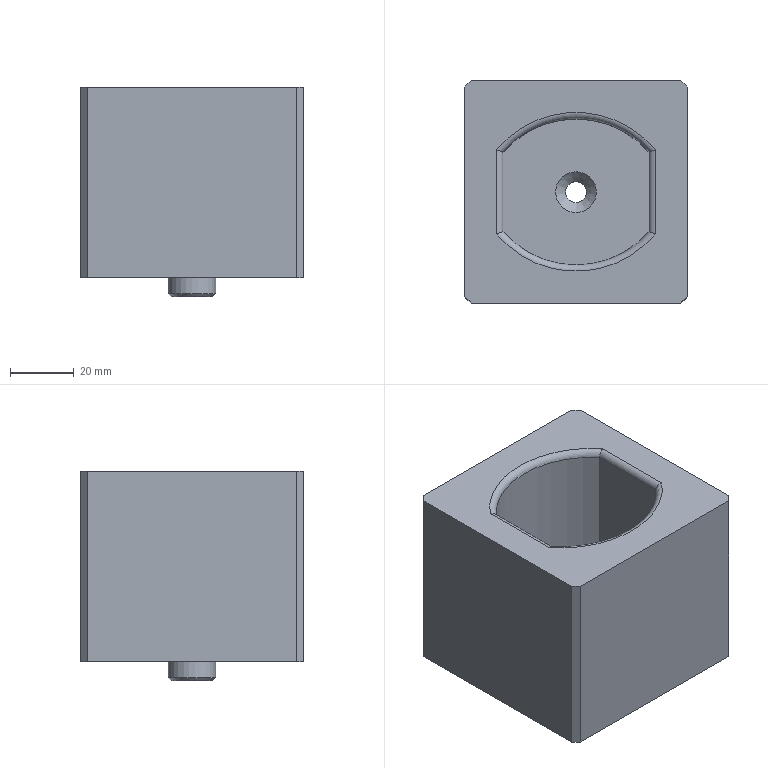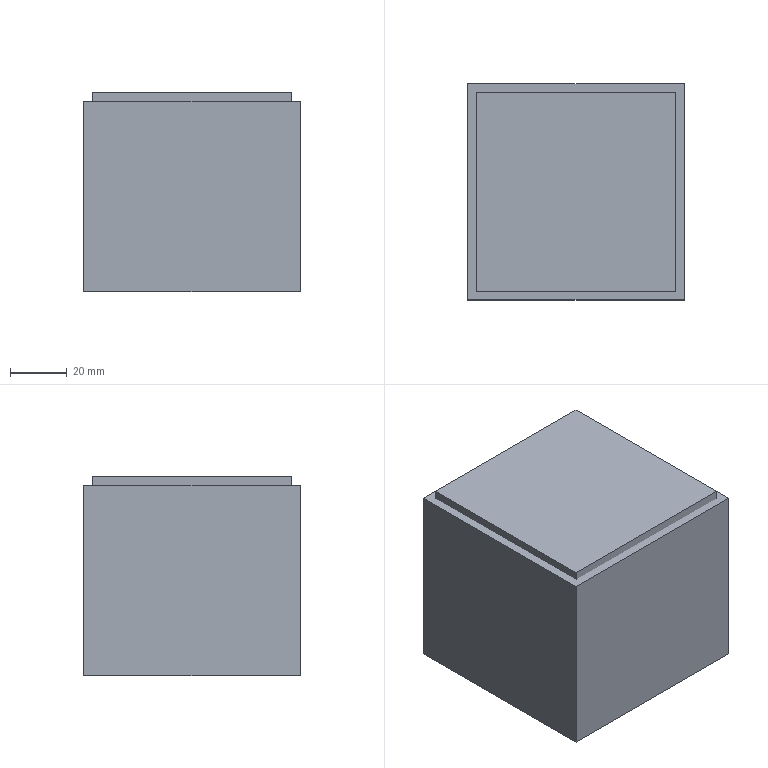CAM job | NX | 3-axis milling, drilling | part box 70 x 70 x 66 mm | stock box 76 x 76 x 70 mm
Tools:
number,name,description,diameter,corner_radius,flute_length,length,flutes
1,D63,Milling Tool-5 Parameters,63.0,0.0,50.0,75.0,2
6,D8A45,Milling Tool-5 Parameters,8.0,0.0,50.0,75.0,2
16,6.6ZT,Drilling Tool,6.6,0.0,35.0,50.0,2
22,D16,Milling Tool-5 Parameters,16.0,0.0,50.0,75.0,2
4,D10,Milling Tool-5 Parameters,10.0,0.0,50.0,75.0,2
18,14.0ZT,Milling Tool-5 Parameters,14.0,0.0,50.0,75.0,2
23,D6R3,Milling Tool-5 Parameters,6.0,3.0,50.0,75.0,2
Operations:
program,operation,operation_type,tool,method,geometry_group,spindle_rpm,surface_speed,feed_per_tooth,feed_cut,feed_plunge,cut_length_mm,path_length_mm,cut_time_min,machine_time_min
1,FLOOR_WALL,VolumeBased25DMillingOperation,D63,METHOD,A,6500.0,1286.0,0.1923,2500.0,100.0,479.797,533.797,0.1919,0.1973
1,DRILLING,Operation,D8A45,METHOD,A,5000.0,0.0,0.0,250.0,0.0,6.4,72.8,0.0256,0.0322
1,DRILLING_COPY,Operation,6.6ZT,METHOD,A,2000.0,41.0,0.0625,250.0,0.0,17.983,95.966,0.0719,0.0797
1,ZLEVEL_PROFILE,ZLevelMilling,D16,METHOD,A,7500.0,376.0,0.1667,2500.0,1000.0,21655.545,21778.745,8.69,8.702
1,ZLEVEL_PROFILE_COPY,ZLevelMilling,D16,METHOD,A,7500.0,376.0,0.0567,850.0,1000.0,1348.483,1540.044,1.583,1.602
1,FLOOR_WALL_1,VolumeBased25DMillingOperation,D10,METHOD,A,7500.0,235.0,0.1667,2500.0,1000.0,6035.627,6237.015,2.448,2.469
1,FLOOR_WALL_1_COPY,VolumeBased25DMillingOperation,D10,METHOD,A,7500.0,235.0,0.0667,1000.0,1000.0,1006.102,1280.289,1.006,1.036
1,PLANAR_MILL,PlanarMilling,D8A45,METHOD,A,7500.0,188.0,0.0833,1250.0,100.0,64.266,121.266,0.0514,0.0571
1,PLANAR_MILL_COPY,PlanarMilling,D8A45,METHOD,A,7500.0,188.0,0.0833,1250.0,100.0,297.482,366.482,0.238,0.2449
2,FLOOR_WALL_COPY,VolumeBased25DMillingOperation,D63,METHOD,B,6500.0,1286.0,0.1923,2500.0,100.0,1823.188,2465.31,0.7293,0.7935
2,ZLEVEL_PROFILE_COPY_1_COPY,ZLevelMilling,D16,METHOD,B,7500.0,376.0,0.1667,2500.0,1000.0,3207.253,3319.303,1.31,1.322
2,ZLEVEL_PROFILE_COPY_1,ZLevelMilling,D16,METHOD,B,7500.0,376.0,0.1667,2500.0,1000.0,5699.6,5811.65,2.307,2.318
2,ZLEVEL_PROFILE_COPY_COPY,ZLevelMilling,D10,METHOD,B,7500.0,376.0,0.0567,850.0,1000.0,784.078,951.443,0.9179,0.9347
2,FLOOR_WALL_1_COPY_COPY,VolumeBased25DMillingOperation,D10,METHOD,B,7500.0,235.0,0.0667,1000.0,1000.0,344.38,511.38,0.3444,0.3611
2,PLANAR_MILL_COPY_COPY,PlanarMilling,D8A45,METHOD,B,7500.0,188.0,0.0833,1250.0,100.0,297.482,354.482,0.238,0.2437
2,DRILLING_COPY_1,Operation,14.0ZT,METHOD,B,3000.0,131.0,0.0417,250.0,0.0,9.4,188.8,0.0376,0.0555
2,ZLEVEL_PROFILE_COPY_1_COPY_COPY,ZLevelMilling,D6R3,METHOD,B,7500.0,376.0,0.1667,2500.0,1000.0,11265.429,11327.629,4.522,4.529